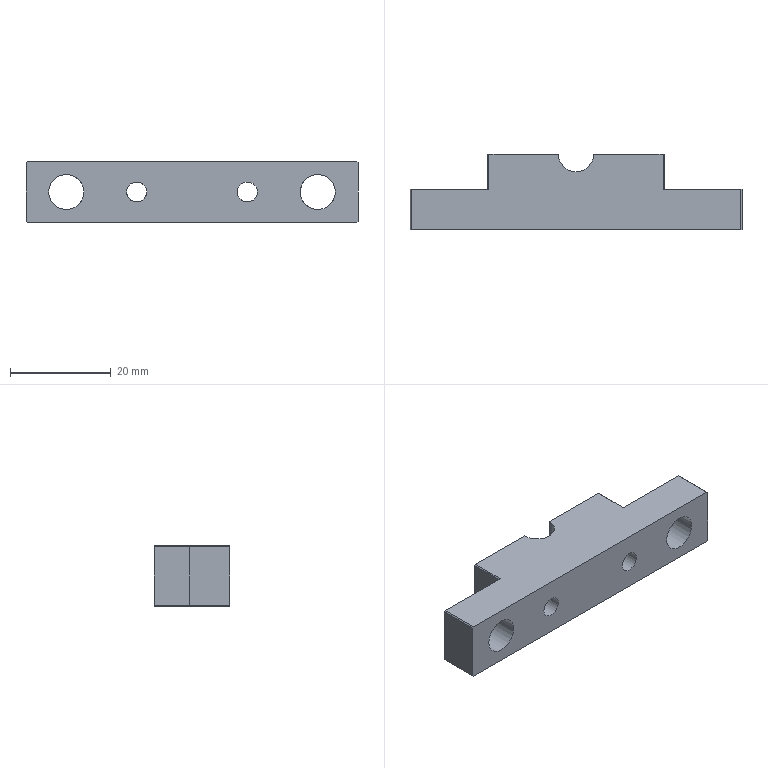NC program | NX | posted with a generic post | part box 66 x 15 x 12 mm
Whole program:
N10 G17 G21 G94 G90
(PLANAR_MILL_2 , TOOL : D10开粗)
N12 T02 M6
N14 G54
N16 G17 G0 G90 X42.8 Y-3. B0. C0. S4500 M3
N18 G43 Z30. H2
N20 Z7.
N22 G94 G1 Z4. F1200.
N24 X32.8
N26 X-32.8
N28 X-42.8
N30 Z7.
N32 G0 Z30.
N34 X42.8 Y3.
N36 Z7.
N38 G1 Z4.
N40 X32.8
N42 X-32.8
N44 X-42.8
N46 Z7.
N48 G0 Z30.
N50 X42.8 Y-3.
N52 Z6.
N54 G1 Z3.
N56 X32.8
N58 X-32.8
N60 X-42.8
N62 Z6.
N64 G0 Z30.
N66 X42.8 Y3.
N68 Z6.
N70 G1 Z3.
N72 X32.8
N74 X-32.8
N76 X-42.8
N78 Z6.
N80 G0 Z30.
N82 X42.8 Y-3.
N84 Z5.
N86 G1 Z2.
N88 X32.8
N90 X-32.8
N92 X-42.8
N94 Z5.
N96 G0 Z30.
N98 X42.8 Y3.
N100 Z5.
N102 G1 Z2.
N104 X32.8
N106 X-32.8
N108 X-42.8
N110 Z5.
N112 G0 Z30.
N114 X42.8 Y-3.
N116 Z4.
N118 G1 Z1.
N120 X32.8
N122 X-32.8
N124 X-42.8
N126 Z4.
N128 G0 Z30.
N130 X42.8 Y3.
N132 Z4.
N134 G1 Z1.
N136 X32.8
N138 X-32.8
N140 X-42.8
N142 Z4.
N144 G0 Z30.
N146 X42.8 Y-3.
N148 Z3.1
N150 G1 Z0.1
N152 X32.8
N154 X-32.8
N156 X-42.8
N158 Z3.1
N160 G0 Z30.
N162 X42.8 Y3.
N164 Z3.1
N166 G1 Z0.1
N168 X32.8
N170 X-32.8
N172 X-42.8
N174 Z3.1
N176 G0 Z30.
(PLANAR_MILL_2_COPY , TOOL : D10开粗)
N178 X42.8 Y-3.
N180 Z3.
N182 G1 Z0. F800.
N184 X32.8
N186 X-32.8
N188 X-42.8
N190 Z3.
N192 G0 Z30.
N194 X42.8 Y3.
N196 Z3.
N198 G1 Z0.
N200 X32.8
N202 X-32.8
N204 X-42.8
N206 Z3.
N208 G0 Z30.
(PLANAR_MILL_3 , TOOL : D10开粗)
N210 X-41. Y0.
N212 Z0.62
N214 G1 Z-1.38 F1200.
N216 X-33.
N218 Y5.8
N220 X-32.8 Y6.
N222 X-24.512
N224 X-21.106 Y9.406
N226 G3 X-22.6 Y5.8 R5.1
N228 G1 Y-5.8
N230 G3 X-21.106 Y-9.406 R5.1
N232 G1 X-24.512 Y-6.
N234 X-32.8
N236 X-33. Y-5.8
N238 Y0.
N240 X-29.
N242 Y2.
N244 X-26.6
N246 Y-2.
N248 X-29.
N250 Y0.
N252 X-37.
N254 Z0.62
N256 G0 Z30.
N258 X-41.
N260 Z-0.76
N262 G1 Z-2.76
N264 X-33.
N266 Y5.8
N268 X-32.8 Y6.
N270 X-24.512
N272 X-21.106 Y9.406
N274 G3 X-22.6 Y5.8 R5.1
N276 G1 Y-5.8
N278 G3 X-21.106 Y-9.406 R5.1
N280 G1 X-24.512 Y-6.
N282 X-32.8
N284 X-33. Y-5.8
N286 Y0.
N288 X-29.
N290 Y2.
N292 X-26.6
N294 Y-2.
N296 X-29.
N298 Y0.
N300 X-37.
N302 Z-0.76
N304 G0 Z30.
N306 X-41.
N308 Z-2.14
N310 G1 Z-4.14
N312 X-33.
N314 Y5.8
N316 X-32.8 Y6.
N318 X-24.512
N320 X-21.106 Y9.406
N322 G3 X-22.6 Y5.8 R5.1
N324 G1 Y-5.8
N326 G3 X-21.106 Y-9.406 R5.1
N328 G1 X-24.512 Y-6.
N330 X-32.8
N332 X-33. Y-5.8
N334 Y0.
N336 X-29.
N338 Y2.
N340 X-26.6
N342 Y-2.
N344 X-29.
N346 Y0.
N348 X-37.
N350 Z-2.14
N352 G0 Z30.
N354 X-41.
N356 Z-3.52
N358 G1 Z-5.52
N360 X-33.
N362 Y5.8
N364 X-32.8 Y6.
N366 X-24.512
N368 X-21.106 Y9.406
N370 G3 X-22.6 Y5.8 R5.1
N372 G1 Y-5.8
N374 G3 X-21.106 Y-9.406 R5.1
N376 G1 X-24.512 Y-6.
N378 X-32.8
N380 X-33. Y-5.8
N382 Y0.
N384 X-29.
N386 Y2.
N388 X-26.6
N390 Y-2.
N392 X-29.
N394 Y0.
N396 X-37.
N398 Z-3.52
N400 G0 Z30.
N402 X-41.
N404 Z-4.9
N406 G1 Z-6.9
N408 X-33.
N410 Y5.8
N412 X-32.8 Y6.
N414 X-24.512
N416 X-21.106 Y9.406
N418 G3 X-22.6 Y5.8 R5.1
N420 G1 Y-5.8
N422 G3 X-21.106 Y-9.406 R5.1
N424 G1 X-24.512 Y-6.
N426 X-32.8
N428 X-33. Y-5.8
N430 Y0.
N432 X-29.
N434 Y2.
N436 X-26.6
N438 Y-2.
N440 X-29.
N442 Y0.
N444 X-37.
N446 Z-4.9
N448 G0 Z30.
N450 X41.
N452 Z0.62
N454 G1 Z-1.38
N456 X33.
N458 Y-5.8
N460 X32.8 Y-6.
N462 X24.512
N464 X21.106 Y-9.406
N466 G3 X22.6 Y-5.8 R5.1
N468 G1 Y5.8
N470 G3 X21.106 Y9.406 R5.1
N472 G1 X24.512 Y6.
N474 X32.8
N476 X33. Y5.8
N478 Y0.
N480 X29.
N482 Y-2.
N484 X26.6
N486 Y2.
N488 X29.
N490 Y0.
N492 X37.
N494 Z0.62
N496 G0 Z30.
N498 X41.
N500 Z-0.76
N502 G1 Z-2.76
N504 X33.
N506 Y-5.8
N508 X32.8 Y-6.
N510 X24.512
N512 X21.106 Y-9.406
N514 G3 X22.6 Y-5.8 R5.1
N516 G1 Y5.8
N518 G3 X21.106 Y9.406 R5.1
N520 G1 X24.512 Y6.
N522 X32.8
N524 X33. Y5.8
N526 Y0.
N528 X29.
N530 Y-2.
N532 X26.6
N534 Y2.
N536 X29.
N538 Y0.
N540 X37.
N542 Z-0.76
N544 G0 Z30.
N546 X41.
N548 Z-2.14
N550 G1 Z-4.14
N552 X33.
N554 Y-5.8
N556 X32.8 Y-6.
N558 X24.512
N560 X21.106 Y-9.406
N562 G3 X22.6 Y-5.8 R5.1
N564 G1 Y5.8
N566 G3 X21.106 Y9.406 R5.1
N568 G1 X24.512 Y6.
N570 X32.8
N572 X33. Y5.8
N574 Y0.
N576 X29.
N578 Y-2.
N580 X26.6
N582 Y2.
N584 X29.
N586 Y0.
N588 X37.
N590 Z-2.14
N592 G0 Z30.
N594 X41.
N596 Z-3.52
N598 G1 Z-5.52
N600 X33.
N602 Y-5.8
N604 X32.8 Y-6.
N606 X24.512
N608 X21.106 Y-9.406
N610 G3 X22.6 Y-5.8 R5.1
N612 G1 Y5.8
N614 G3 X21.106 Y9.406 R5.1
N616 G1 X24.512 Y6.
N618 X32.8
N620 X33. Y5.8
N622 Y0.
N624 X29.
N626 Y-2.
N628 X26.6
N630 Y2.
N632 X29.
N634 Y0.
N636 X37.
N638 Z-3.52
N640 G0 Z30.
N642 X41.
N644 Z-4.9
N646 G1 Z-6.9
N648 X33.
N650 Y-5.8
N652 X32.8 Y-6.
N654 X24.512
N656 X21.106 Y-9.406
N658 G3 X22.6 Y-5.8 R5.1
N660 G1 Y5.8
N662 G3 X21.106 Y9.406 R5.1
N664 G1 X24.512 Y6.
N666 X32.8
N668 X33. Y5.8
N670 Y0.
N672 X29.
N674 Y-2.
N676 X26.6
N678 Y2.
N680 X29.
N682 Y0.
N684 X37.
N686 Z-4.9
N688 G0 Z30.
(PLANAR_MILL_3_COPY , TOOL : D10开粗)
N690 X-41.
N692 Z-5.
N694 G1 Z-7. F800.
N696 X-33.
N698 Y5.8
N700 X-32.8 Y6.
N702 X-24.371
N704 X-21.036 Y9.336
N706 G3 X-22.5 Y5.8 R5.
N708 G1 Y-5.8
N710 G3 X-21.036 Y-9.336 R5.
N712 G1 X-24.371 Y-6.
N714 X-32.8
N716 X-33. Y-5.8
N718 Y0.
N720 X-29.
N722 Y2.
N724 X-26.5
N726 Y-2.
N728 X-29.
N730 Y0.
N732 X-37.
N734 Z-5.
N736 G0 Z30.
N738 X41.
N740 Z-5.
N742 G1 Z-7.
N744 X33.
N746 Y-5.8
N748 X32.8 Y-6.
N750 X24.371
N752 X21.036 Y-9.336
N754 G3 X22.5 Y-5.8 R5.
N756 G1 Y5.8
N758 G3 X21.036 Y9.336 R5.
N760 G1 X24.371 Y6.
N762 X32.8
N764 X33. Y5.8
N766 Y0.
N768 X29.
N770 Y-2.
N772 X26.5
N774 Y2.
N776 X29.
N778 Y0.
N780 X37.
N782 Z-5.
N784 G0 Z30.
(PLANAR_MILL_3_COPY_COPY , TOOL : D10开粗)
N786 X-15.886 Y-14.485
N788 Z-5.
N790 G1 Z-7.
N792 X-20.836 Y-9.536
N794 X-21.036 Y-9.336
N796 G2 X-22.5 Y-5.8 R5.
N798 G1 Y5.8
N800 G2 X-21.036 Y9.336 R5.
N802 G1 X-20.836 Y9.536
N804 X-15.886 Y14.485
N806 Z-5.
N808 G0 Z30.
N810 X15.886
N812 Z-5.
N814 G1 Z-7.
N816 X20.836 Y9.536
N818 X21.036 Y9.336
N820 G2 X22.5 Y5.8 R5.
N822 G1 Y-5.8
N824 G2 X21.036 Y-9.336 R5.
N826 G1 X20.836 Y-9.536
N828 X15.886 Y-14.485
N830 Z-5.
N832 G0 Z30.
N834 M5
(DRILLING_1 , TOOL : D8倒角刀)
N836 T04 M6
N838 G54
N840 G17 G0 G90 X-11. Y0. B0. C0. S3000 M3
N842 G43 Z30. H4
N844 G94 G81 G98 Z-2.1 F200. R3.
N846 X11.
N848 G80
N850 G0 X11. Y0. Z30.
(DRILLING_1_COPY , TOOL : D8倒角刀)
N852 X-25.
N854 G81 Z-10.5 F200. R-4.
N856 X25.
N858 G80
N860 G0 X25. Y0. Z30.
(PLANAR_MILL_4 , TOOL : D8倒角刀)
N862 X0. Y-11.5 S3500
N864 Z1.5
N866 G1 Z-1.5 F1000.
N868 Y-7.5
N870 X-17.3
N872 G2 X-18.361 Y-7.061 R1.5
N874 G1 X-18.561 Y-6.861
N876 G2 X-19. Y-5.8 R1.5
N878 G1 Y5.8
N880 G2 X-18.561 Y6.861 R1.5
N882 G1 X-18.361 Y7.061
N884 G2 X-17.3 Y7.5 R1.5
N886 G1 X17.3
N888 G2 X18.361 Y7.061 R1.5
N890 G1 X18.561 Y6.861
N892 G2 X19. Y5.8 R1.5
N894 G1 Y-5.8
N896 G2 X18.561 Y-6.861 R1.5
N898 G1 X18.361 Y-7.061
N900 G2 X17.3 Y-7.5 R1.5
N902 G1 X0.
N904 Y-11.5
N906 Z1.5
N908 G0 Z30.
N910 M5
(CURVE_DRIVE , TOOL : R1)
N912 T08 M6
N914 G54
N916 G17 G0 G90 X2.498 Y7.045 B0. C0. S5500 M3
N918 G43 Z30. H8
N920 Z2.725
N922 G94 G1 Z-0.168 F2000.
N924 Y7.028 Z-0.31
N926 Y6.992 Z-0.447
N928 X2.497 Y6.936 Z-0.579
N930 Y6.861 Z-0.701
N932 Y6.771 Z-0.811
N934 Y6.665 Z-0.907
N936 Y6.547 Z-0.987
N938 Y6.419 Z-1.05
N940 Y6.283 Z-1.093
N942 X2.496 Y6.142 Z-1.117
N944 Y6. Z-1.121
N946 Y5.995 Z-1.12
N948 Y5.973 Z-1.113
N950 X2.497 Y5.954 Z-1.091
N952 Y5.949 Z-1.081
N954 X2.498 Y5.93 Z-1.05
N956 Y-5.945
N958 X2.497 Y-5.96 Z-1.097
N960 X2.496 Y-5.975 Z-1.111
N962 Y-6. Z-1.117
N964 Z-1.138
N966 X2.494 Z-1.158
N968 Y-5.949 Z-1.153
N970 X2.496 Y-5.926 Z-1.134
N972 Y-5.913 Z-1.114
N974 X2.497 Y-5.9 Z-1.1
N976 Y5.849
N978 Y5.903 Z-1.102
N980 X2.496 Y5.925 Z-1.134
N982 X2.494 Y5.937 Z-1.148
N984 Y5.949 Z-1.153
N986 Y6. Z-1.158
N988 Y5.949 Z-1.153
N990 Y5.941 Z-1.15
N992 Y-5.945
N994 Y-5.949 Z-1.153
N996 Y-6. Z-1.158
N998 X2.489 Z-1.204
N1000 Y-5.949 Z-1.2
N1002 Y5.949
N1004 Y6. Z-1.204
N1006 X2.484 Z-1.253
N1008 Y5.98 Z-1.252
N1010 Y5.949 Z-1.249
N1012 Y-5.949
N1014 Y-5.98 Z-1.252
N1016 Y-6. Z-1.253
N1018 X2.479 Z-1.302
N1020 Y-5.949 Z-1.299
N1022 Y5.949
N1024 Y6. Z-1.302
N1026 X2.477 Z-1.322
N1028 X2.472 Z-1.351
N1030 Y5.949 Z-1.349
N1032 Y-5.949
N1034 Y-6. Z-1.351
N1036 X2.465 Z-1.4
N1038 Y-5.949 Z-1.398
N1040 Y5.949
N1042 Y6. Z-1.4
N1044 X2.457 Z-1.449
N1046 Y5.949 Z-1.448
N1048 Y-5.95
N1050 Y-6. Z-1.449
N1052 X2.447 Z-1.497
N1054 Y-5.986
N1056 Y-5.949 Z-1.496
N1058 Y5.949
N1060 Y5.986 Z-1.497
N1062 Y6.
N1064 X2.437 Z-1.547
N1066 Y5.985 Z-1.544
N1068 Y5.949 Z-1.545
N1070 Y-5.949
N1072 Y-5.985 Z-1.544
N1074 Y-6. Z-1.547
N1076 X2.427 Z-1.596
N1078 Y-5.966 Z-1.588
N1080 Y-5.949 Z-1.589
N1082 Y5.949
N1084 Y5.968 Z-1.588
N1086 Y6. Z-1.596
N1088 X2.419 Z-1.632
N1090 X2.416 Z-1.643
N1092 Y5.949 Z-1.637
N1094 Y-5.949
N1096 Y-6. Z-1.643
N1098 X2.402 Z-1.691
N1100 Y-5.949 Z-1.685
N1102 Y5.949
N1104 Y6. Z-1.691
N1106 X2.387 Z-1.739
N1108 Y5.949 Z-1.733
N1110 Y-5.949 Z-1.732
N1112 Y-6. Z-1.739
N1114 X2.381 Z-1.761
N1116 X2.372 Z-1.784
N1118 Y-5.958 Z-1.779
N1120 Y-5.949 Z-1.78
N1122 Y5.949
N1124 Y5.958 Z-1.779
N1126 Y6. Z-1.784
N1128 X2.356 Z-1.827
N1130 Y5.974 Z-1.823
N1132 Y5.949 Z-1.827
N1134 Y-5.949
N1136 Y-5.974 Z-1.823
N1138 Y-6. Z-1.827
N1140 X2.339 Z-1.87
N1142 Y-5.991 Z-1.868
N1144 Y-5.955 Z-1.874
N1146 Y5.955
N1148 Y5.991 Z-1.869
N1150 Y6. Z-1.87
N1152 X2.33 Z-1.894
N1154 X2.323 Z-1.915
N1156 Y5.988 Z-1.917
N1158 Y5.949 Z-1.916
N1160 Y-5.949
N1162 Y-5.988 Z-1.917
N1164 Y-6. Z-1.915
N1166 X2.317 Z-1.932
N1168 X2.305 Z-1.962
N1170 Y-5.949
N1172 Y5.949
N1174 Y6.
N1176 X2.285 Z-2.008
N1178 Y5.989 Z-2.007
N1180 Y5.949
N1182 Y-5.949
N1184 Y-5.989
N1186 Y-6. Z-2.008
N1188 X2.266 Z-2.054
N1190 Y-5.95 Z-2.05
N1192 Y5.95
N1194 Y6. Z-2.054
N1196 X2.244 Z-2.099
N1198 Y5.949 Z-2.095
N1200 Y-5.949
N1202 Y-6. Z-2.099
N1204 X2.222 Z-2.144
N1206 Y-5.949 Z-2.14
N1208 Y5.949
N1210 Y6. Z-2.144
N1212 X2.199 Z-2.188
N1214 Y5.949 Z-2.184
N1216 Y-5.949
N1218 Y-6. Z-2.188
N1220 X2.189 Z-2.209
N1222 X2.175 Z-2.23
N1224 Y-5.977 Z-2.228
N1226 Y5.977
N1228 Y6. Z-2.23
N1230 X2.163 Z-2.248
N1232 X2.149 Z-2.272
N1234 Y5.949 Z-2.271
N1236 Y-5.949
N1238 Y-6. Z-2.272
N1240 X2.137 Z-2.292
N1242 X2.124 Z-2.313
N1244 Y-5.973 Z-2.314
N1246 Y5.973
N1248 Y6. Z-2.313
N1250 X2.098 Z-2.356
N1252 Y5.974 Z-2.354
N1254 Y5.949 Z-2.355
N1256 Y-5.949
N1258 Y-5.974 Z-2.354
N1260 Y-6. Z-2.356
N1262 X2.072 Z-2.398
N1264 Y-5.951 Z-2.395
N1266 Y5.95
N1268 Y6. Z-2.398
N1270 X2.043 Z-2.438
N1272 Y5.98 Z-2.436
N1274 Y-5.98
N1276 Y-6. Z-2.437
N1278 X2.014 Z-2.477
N1280 Y-5.206
N1282 Y5.949
N1284 Y6.
N1286 X1.997 Z-2.501
N1288 X1.984 Z-2.517
N1290 Y5.956 Z-2.516
N1292 Y5.949 Z-2.517
N1294 Y-5.949
N1296 Y-5.956 Z-2.516
N1298 Y-6. Z-2.517
N1300 X1.953 Z-2.555
N1302 Y-5.971 Z-2.554
N1304 Y-5.949 Z-2.556
N1306 Y5.949
N1308 Y5.971 Z-2.554
N1310 Y6. Z-2.555
N1312 X1.921 Z-2.593
N1314 Y5.987
N1316 Y5.949 Z-2.595
N1318 Y-5.949
N1320 Y-5.987 Z-2.593
N1322 Y-6.
N1324 X1.89 Z-2.631
N1326 Y-5.979 Z-2.632
N1328 Y5.979
N1330 Y6. Z-2.631
N1332 X1.858 Z-2.67
N1334 Y-6.
N1336 X1.843 Z-2.688
N1338 X1.825 Z-2.706
N1340 Y6.
N1342 X1.817 Z-2.715
N1344 X1.791 Z-2.743
N1346 Y5.974 Z-2.741
N1348 Y-5.974
N1350 Y-6. Z-2.743
N1352 X1.755 Z-2.778
N1354 Y-5.949 Z-2.776
N1356 Y5.96
N1358 Y6. Z-2.778
N1360 X1.72 Z-2.812
N1362 Y5.949 Z-2.811
N1364 Y-5.996
N1366 Y-6. Z-2.812
N1368 X1.689 Z-2.842
N1370 X1.684 Z-2.846
N1372 Y6.
N1374 X1.646 Z-2.879
N1376 Y-6.
N1378 X1.608 Z-2.911
N1380 Y6.
N1382 X1.57 Z-2.943
N1384 Y-6.
N1386 X1.536 Z-2.972
N1388 X1.531 Z-2.975
N1390 Y6.
N1392 X1.491 Z-3.004
N1394 Y-6.
N1396 X1.45 Z-3.033
N1398 Y6.
N1400 X1.409 Z-3.062
N1402 Y-6.
N1404 X1.368 Z-3.091
N1406 Y-5.977
N1408 Y-5.956 Z-3.09
N1410 Y5.956
N1412 Y5.977 Z-3.091
N1414 Y6.
N1416 X1.357 Z-3.099
N1418 X1.326 Z-3.117
N1420 Y5.978 Z-3.116
N1422 Y5.949
N1424 Y-5.949
N1426 Y-5.978
N1428 Y-6. Z-3.117
N1430 X1.283 Z-3.142
N1432 Y-5.949
N1434 Y5.971
N1436 Y6.
N1438 X1.241 Z-3.168
N1440 Y-6.
N1442 X1.202 Z-3.189
N1444 X1.197 Z-3.192
N1446 Y6.
N1448 X1.153 Z-3.215
N1450 Y5.95 Z-3.216
N1452 Y-5.95
N1454 Y-6. Z-3.215
N1456 X1.109 Z-3.238
N1458 Y6.
N1460 X1.064 Z-3.26
N1462 Y-6.
N1464 X1.049 Z-3.267
N1466 X1.019 Z-3.28
N1468 Y-5.97 Z-3.281
N1470 Y5.97
N1472 Y6. Z-3.28
N1474 X0.973 Z-3.3
N1476 Y5.975 Z-3.301
N1478 Y-5.975
N1480 Y-6. Z-3.3
N1482 X0.948 Z-3.311
N1484 X0.927 Z-3.319
N1486 Y6.
N1488 X0.88 Z-3.337
N1490 Y-6.
N1492 X0.833 Z-3.354
N1494 Y-5.949 Z-3.355
N1496 Y5.961
N1498 Y6. Z-3.354
N1500 X0.786 Z-3.371
N1502 Y-6.
N1504 X0.768 Z-3.377
N1506 X0.739 Z-3.386
N1508 X0.738 Y6.
N1510 X0.691 Z-3.4
N1512 Y-6.
N1514 X0.643 Z-3.414
N1516 Y6.
N1518 X0.614 Z-3.423
N1520 X0.594 Z-3.427
N1522 Y-6.
N1524 X0.545 Z-3.437
N1526 Y6.
N1528 X0.496 Z-3.447
N1530 Y-6.
N1532 X0.447 Z-3.457
N1534 Y6.
N1536 X0.398 Z-3.465
N1538 Y5.949 Z-3.466
N1540 Y-5.963
N1542 Y-6. Z-3.465
N1544 X0.349 Z-3.473
N1546 Y6.
N1548 X0.299 Z-3.479
N1550 Y-6.
N1552 X0.249 Z-3.484
N1554 Y6.
N1556 X0.2 Z-3.49
N1558 Y-6.
N1560 X0.15 Z-3.495
N1562 Y6.
N1564 X0.1 Z-3.497
N1566 Y-6.
N1568 X0.05 Z-3.498
N1570 Y6.
N1572 X0. Z-3.5
N1574 Y-6.
N1576 X-0.05 Z-3.498
N1578 Y-5.949 Z-3.499
N1580 Y5.949
N1582 Y6. Z-3.498
N1584 X-0.1 Z-3.497
N1586 Y5.949
N1588 Y-5.972
N1590 Y-6.
N1592 X-0.15 Z-3.495
N1594 Y6.
N1596 X-0.2 Z-3.49
N1598 Y-6.
N1600 X-0.249 Z-3.484
N1602 Y6.
N1604 X-0.299 Z-3.479
N1606 Y-6.
N1608 X-0.349 Z-3.473
N1610 Y6.
N1612 X-0.398 Z-3.465
N1614 Y5.949 Z-3.466
N1616 Y-5.963
N1618 Y-6. Z-3.465
N1620 X-0.447 Z-3.457
N1622 Y6.
N1624 X-0.496 Z-3.447
N1626 Y-6.
N1628 X-0.545 Z-3.437
N1630 Y6.
N1632 X-0.594 Z-3.427
N1634 Y-6.
N1636 X-0.614 Z-3.423
N1638 X-0.642 Z-3.414
N1640 Y6.
N1642 X-0.69 Z-3.4
N1644 Y-6.
N1646 X-0.738 Z-3.386
N1648 Y6.
N1650 X-0.768 Z-3.377
N1652 X-0.786 Z-3.371
N1654 Y-6.
N1656 X-0.833 Z-3.354
N1658 Y-5.949 Z-3.355
N1660 Y5.961
N1662 Y6. Z-3.354
N1664 X-0.88 Z-3.337
N1666 Y-6.
N1668 X-0.926 Z-3.319
N1670 Y6.
N1672 X-0.948 Z-3.311
N1674 X-0.973 Z-3.3
N1676 Y5.975 Z-3.301
N1678 Y-5.975
N1680 Y-6. Z-3.3
N1682 X-1.018 Z-3.28
N1684 Y-5.969 Z-3.281
N1686 Y5.969
N1688 Y6. Z-3.28
N1690 X-1.049 Z-3.267
N1692 X-1.063 Z-3.26
N1694 Y-6.
N1696 X-1.108 Z-3.238
N1698 Y6.
N1700 X-1.153 Z-3.215
N1702 Y5.949 Z-3.216
N1704 Y-5.95
N1706 Y-6. Z-3.215
N1708 X-1.197 Z-3.192
N1710 Y6.
N1712 X-1.229 Z-3.175
N1714 X-1.24 Z-3.168
N1716 Y-6.
N1718 X-1.283 Z-3.142
N1720 Y-5.949
N1722 Y5.972
N1724 Y6.
N1726 X-1.326 Z-3.117
N1728 Y5.978 Z-3.116
N1730 Y5.949
N1732 Y-5.949
N1734 Y-5.978
N1736 Y-6. Z-3.117
N1738 X-1.357 Z-3.099
N1740 X-1.368 Z-3.091
N1742 Y-5.978
N1744 Y-5.956 Z-3.09
N1746 Y5.956
N1748 Y5.978 Z-3.091
N1750 Y6.
N1752 X-1.409 Z-3.062
N1754 Y-6.
N1756 X-1.45 Z-3.033
N1758 Y6.
N1760 X-1.49 Z-3.004
N1762 Y-6.
N1764 X-1.531 Z-2.975
N1766 Y6.
N1768 X-1.536 Z-2.972
N1770 X-1.569 Z-2.943
N1772 Y-6.
N1774 X-1.608 Z-2.911
N1776 Y6.
N1778 X-1.646 Z-2.879
N1780 Y-6.
N1782 X-1.684 Z-2.846
N1784 Y6.
N1786 X-1.689 Z-2.842
N1788 X-1.72 Z-2.812
N1790 Y5.949 Z-2.811
N1792 Y-5.996 Z-2.812
N1794 Y-6.
N1796 X-1.755 Z-2.778
N1798 Y-5.96 Z-2.776
N1800 Y5.96
N1802 Y6. Z-2.778
N1804 X-1.79 Z-2.744
N1806 Y5.973 Z-2.741
N1808 Y-5.973
N1810 Y-6. Z-2.744
N1812 X-1.817 Z-2.714
N1814 X-1.824 Z-2.707
N1816 Y6.
N1818 X-1.843 Z-2.688
N1820 X-1.858 Z-2.67
N1822 Y-6.
N1824 X-1.89 Z-2.631
N1826 Y-5.979 Z-2.633
N1828 Y5.979
N1830 Y6. Z-2.631
N1832 X-1.921 Z-2.593
N1834 Y5.987
N1836 Y5.949 Z-2.595
N1838 Y-5.949
N1840 Y-5.987 Z-2.593
N1842 Y-6.
N1844 X-1.952 Z-2.555
N1846 Y-5.972
N1848 Y-5.949 Z-2.556
N1850 Y5.949
N1852 Y5.971 Z-2.555
N1854 Y6.
N1856 X-1.983 Z-2.517
N1858 Y5.956
N1860 Y5.949
N1862 Y-5.949
N1864 Y-5.956
N1866 Y-6.
N1868 X-1.997 Z-2.501
N1870 X-2.013 Z-2.478
N1872 Y-5.206 Z-2.477
N1874 Y5.949
N1876 Y6. Z-2.478
N1878 X-2.042 Z-2.438
N1880 Y5.98 Z-2.437
N1882 Y-5.98
N1884 Y-6. Z-2.438
N1886 X-2.071 Z-2.399
N1888 Y-5.951 Z-2.396
N1890 Y5.951
N1892 Y6. Z-2.399
N1894 X-2.098 Z-2.356
N1896 Y5.973 Z-2.355
N1898 Y5.949 Z-2.356
N1900 Y-5.949
N1902 Y-5.973 Z-2.355
N1904 Y-6. Z-2.356
N1906 X-2.123 Z-2.313
N1908 Y-5.972 Z-2.315
N1910 Y5.972
N1912 Y6. Z-2.313
N1914 X-2.138 Z-2.291
N1916 X-2.149 Z-2.272
N1918 Y5.949
N1920 Y-5.949
N1922 Y-6.
N1924 X-2.163 Z-2.248
N1926 X-2.175 Z-2.23
N1928 Y-5.977 Z-2.229
N1930 Y5.977
N1932 Y6. Z-2.23
N1934 X-2.189 Z-2.209
N1936 X-2.199 Z-2.189
N1938 Y5.949 Z-2.185
N1940 Y-5.949
N1942 Y-6. Z-2.189
N1944 X-2.222 Z-2.145
N1946 Y-5.949 Z-2.141
N1948 Y5.949
N1950 Y6. Z-2.145
N1952 X-2.244 Z-2.1
N1954 Y5.949 Z-2.096
N1956 Y-5.949
N1958 Y-6. Z-2.1
N1960 X-2.266 Z-2.055
N1962 Y-5.95 Z-2.051
N1964 Y5.95
N1966 Y6. Z-2.055
N1968 X-2.285 Z-2.009
N1970 Y5.989 Z-2.008
N1972 Y5.949 Z-2.007
N1974 Y-5.949
N1976 Y-5.989 Z-2.008
N1978 Y-6. Z-2.009
N1980 X-2.305 Z-1.963
N1982 Y-5.949 Z-1.962
N1984 Y5.949
N1986 Y6. Z-1.963
N1988 X-2.317 Z-1.932
N1990 X-2.323 Z-1.916
N1992 Y5.989 Z-1.918
N1994 Y5.949 Z-1.917
N1996 Y-5.949
N1998 Y-5.989 Z-1.918
N2000 Y-6. Z-1.916
N2002 X-2.33 Z-1.894
N2004 X-2.339 Z-1.87
N2006 Y-5.991 Z-1.869
N2008 Y-5.956 Z-1.875
N2010 Y5.956
N2012 Y5.991 Z-1.869
N2014 Y6. Z-1.87
N2016 X-2.355 Z-1.827
N2018 Y5.974 Z-1.824
N2020 Y5.949 Z-1.828
N2022 Y-5.949
N2024 Y-5.974 Z-1.824
N2026 Y-6. Z-1.827
N2028 X-2.372 Z-1.785
N2030 Y-5.958 Z-1.779
N2032 Y-5.949 Z-1.781
N2034 Y5.949
N2036 Y5.958 Z-1.779
N2038 Y6. Z-1.785
N2040 X-2.381 Z-1.761
N2042 X-2.387 Z-1.74
N2044 Y5.949 Z-1.733
N2046 Y-5.949
N2048 Y-6. Z-1.74
N2050 X-2.401 Z-1.692
N2052 Y-5.949 Z-1.685
N2054 Y5.949
N2056 Y6. Z-1.692
N2058 X-2.416 Z-1.644
N2060 Y5.949 Z-1.637
N2062 Y-5.949
N2064 Y-6. Z-1.644
N2066 X-2.419 Z-1.632
N2068 X-2.427 Z-1.599
N2070 Y-5.965 Z-1.59
N2072 Y-5.949 Z-1.591
N2074 Y5.949
N2076 Y5.966
N2078 Y6. Z-1.599
N2080 X-2.437 Z-1.548
N2082 Y5.985 Z-1.545
N2084 Y5.949 Z-1.547
N2086 Y-5.949
N2088 Y-5.985 Z-1.545
N2090 Y-6. Z-1.548
N2092 X-2.447 Z-1.498
N2094 Y-5.984 Z-1.499
N2096 Y-5.949 Z-1.498
N2098 Y5.949
N2100 Y5.984 Z-1.499
N2102 Y6. Z-1.498
N2104 X-2.457 Z-1.45
N2106 Y5.949 Z-1.449
N2108 Y-5.949
N2110 Y-6. Z-1.45
N2112 X-2.465 Z-1.402
N2114 Y-5.949 Z-1.4
N2116 Y5.949
N2118 Y6. Z-1.402
N2120 X-2.472 Z-1.353
N2122 Y5.949 Z-1.35
N2124 Y-5.949
N2126 Y-6. Z-1.353
N2128 X-2.477 Z-1.32
N2130 X-2.478 Z-1.303
N2132 Y-5.949 Z-1.301
N2134 Y5.949 Z-1.3
N2136 Y6. Z-1.303
N2138 X-2.484 Z-1.255
N2140 Y5.979 Z-1.253
N2142 Y5.949 Z-1.251
N2144 Y-5.949
N2146 Y-5.979 Z-1.254
N2148 Y-6. Z-1.255
N2150 X-2.489 Z-1.206
N2152 Y-5.949 Z-1.201
N2154 Y5.949
N2156 Y6. Z-1.206
N2158 X-2.494 Z-1.156
N2160 Y5.949 Z-1.151
N2162 Y-5.949
N2164 Y-6. Z-1.156
N2166 X-2.496 Z-1.138
N2168 X-2.497 Z-1.106
N2170 Y-5.949 Z-1.101
N2172 Y5.949
N2174 Y6. Z-1.106
N2176 X-2.498 Z-1.068
N2178 Y5.999 Z-1.055
N2180 Y5.949 Z-1.051
N2182 Y-5.956 Z-1.052
N2184 Y-5.992 Z-1.055
N2186 X-2.5 Y-5.965 Z-1.002
N2188 Y-5.949 Z-1.001
N2190 Y5.95
N2192 Y5.993 Z-1.005
N2194 X-2.504 Y6.136 Z-1.007
N2196 X-2.507 Y6.277 Z-0.988
N2198 X-2.51 Y6.415 Z-0.95
N2200 X-2.513 Y6.545 Z-0.893
N2202 X-2.516 Y6.666 Z-0.817
N2204 X-2.519 Y6.775 Z-0.725
N2206 X-2.521 Y6.87 Z-0.619
N2208 X-2.523 Y6.949 Z-0.5
N2210 X-2.524 Y7.01 Z-0.371
N2212 X-2.525 Y7.052 Z-0.234
N2214 X-2.526 Y7.074 Z-0.093
N2216 Z2.724
N2218 G0 Z30.
N2220 M5
N2222 M2